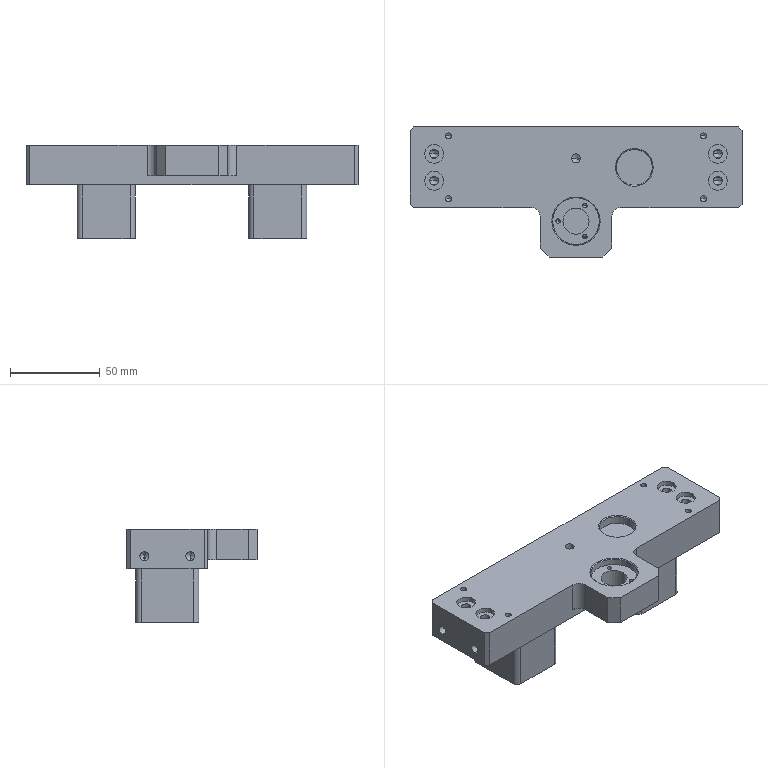NC program | NX | posted with a generic post | part box 185 x 72.5 x 52 mm
Lines 6548 to 6926 of 6926:
(ZLEVEL_PROFILE_COPY_1_COPY_COPY_1 , TOOL : D10JING)
N13076 T14 M6
N13078 G54
N13080 G17 G0 G90 X-32.847 Y-38.112 S9500 M3
N13082 G43 Z30. H14
N13084 Z-13.5
N13086 G94 G1 Z-14.5 F1000.
N13088 X-33.634 Y-36.75
N13090 G3 X-34.5 Y-36.25 R1.
N13092 G1 X-61. F1200.
N13094 G2 X-69. Y-28.25 R8.
N13096 G1 Y0.75
N13098 G2 X-61. Y8.75 R8.
N13100 G1 X-34.5
N13102 G2 X-26.5 Y0.75 R8.
N13104 G1 Y-28.25
N13106 G2 X-34.5 Y-36.25 R8.
N13108 G3 X-35.366 Y-36.75 R1.
N13110 G1 X-36.232 Y-38.25
N13112 Z-13.5
N13114 G0 Z30.
N13116 X-32.847 Y-38.112
N13118 Z-28.
N13120 G1 Z-29. F1000.
N13122 X-33.634 Y-36.75
N13124 G3 X-34.5 Y-36.25 R1.
N13126 G1 X-61. F1200.
N13128 G2 X-69. Y-28.25 R8.
N13130 G1 Y0.75
N13132 G2 X-61. Y8.75 R8.
N13134 G1 X-34.5
N13136 G2 X-26.5 Y0.75 R8.
N13138 G1 Y-28.25
N13140 G2 X-34.5 Y-36.25 R8.
N13142 G3 X-35.366 Y-36.75 R1.
N13144 G1 X-36.232 Y-38.25
N13146 Z-28.
N13148 G0 Z30.
N13150 X62.653 Y-38.112
N13152 Z-13.5
N13154 G1 Z-14.5 F1000.
N13156 X61.866 Y-36.75
N13158 G3 X61. Y-36.25 R1.
N13160 G1 X34.5 F1200.
N13162 G2 X26.5 Y-28.25 R8.
N13164 G1 Y0.75
N13166 G2 X34.5 Y8.75 R8.
N13168 G1 X61.
N13170 G2 X69. Y0.75 R8.
N13172 G1 Y-28.25
N13174 G2 X61. Y-36.25 R8.
N13176 G3 X60.134 Y-36.75 R1.
N13178 G1 X59.268 Y-38.25
N13180 Z-13.5
N13182 G0 Z30.
N13184 X62.653 Y-38.112
N13186 Z-28.
N13188 G1 Z-29. F1000.
N13190 X61.866 Y-36.75
N13192 G3 X61. Y-36.25 R1.
N13194 G1 X34.5 F1200.
N13196 G2 X26.5 Y-28.25 R8.
N13198 G1 Y0.75
N13200 G2 X34.5 Y8.75 R8.
N13202 G1 X61.
N13204 G2 X69. Y0.75 R8.
N13206 G1 Y-28.25
N13208 G2 X61. Y-36.25 R8.
N13210 G3 X60.134 Y-36.75 R1.
N13212 G1 X59.268 Y-38.25
N13214 Z-28.
N13216 G0 Z30.
(ZLEVEL_PROFILE_COPY_1_COPY_COPY_1_COPY , TOOL : D10JING)
N13218 X92.122 Y-43.059
N13220 Z-51.
N13222 G1 Z-52. F1000.
N13224 X91.366 Y-41.75
N13226 G3 X90.5 Y-41.25 R1.
N13228 G1 X-90.5 F1200.
N13230 G2 X-94.036 Y-39.786 R5.
N13232 G1 X-96.036 Y-37.786
N13234 G2 X-97.5 Y-34.25 R5.
N13236 G1 Y6.75
N13238 G2 X-96.036 Y10.286 R5.
N13240 G1 X-94.036 Y12.286
N13242 G2 X-90.5 Y13.75 R5.
N13244 G1 X-25.
N13246 Y31.25
N13248 G2 X-23.536 Y34.786 R5.
N13250 G1 X-18.536 Y39.786
N13252 G2 X-15. Y41.25 R5.
N13254 G1 X15.
N13256 G2 X18.536 Y39.786 R5.
N13258 G1 X23.536 Y34.786
N13260 G2 X25. Y31.25 R5.
N13262 G1 Y13.75
N13264 X90.5
N13266 G2 X94.036 Y12.286 R5.
N13268 G1 X96.036 Y10.286
N13270 G2 X97.5 Y6.75 R5.
N13272 G1 Y-34.25
N13274 G2 X96.036 Y-37.786 R5.
N13276 G1 X94.036 Y-39.786
N13278 G2 X90.5 Y-41.25 R5.
N13280 G3 X89.634 Y-41.75 R1.
N13282 G1 X88.768 Y-43.25
N13284 Z-51.
N13286 G0 Z30.
(FLOOR_WALL , TOOL : D10JING)
N13288 X93.714 Y-42.229
N13290 Z-28.5
N13292 G1 Z-30. F1250.
N13294 X93.437 Y-41.75
N13296 G3 X92.571 Y-41.25 R1.
N13298 G1 X-92.571
N13300 X-97.171 Y-36.65
N13302 X-62.3
N13304 G2 X-68.603 Y-32.05 R8.5
N13306 G1 X-97.5
N13308 Y-27.45
N13310 X-69.5
N13312 Y-22.85
N13314 X-97.5
N13316 Y-18.25
N13318 X-69.5
N13320 Y-13.65
N13322 X-97.5
N13324 Y-9.05
N13326 X-69.5
N13328 Y-4.45
N13330 X-97.5
N13332 Y0.15
N13334 X-69.5
N13336 Y0.75
N13338 G2 X-68.5 Y4.75 R8.5
N13340 G1 X-97.5
N13342 G3 X-98.366 Y4.25 R1.
N13344 G1 X-99. Y3.152
N13346 Z-28.5
N13348 G0 Z30.
N13350 X68.271 Y-36.65
N13352 Z-28.4
N13354 G1 X62.3 Z-30.
N13356 X97.171
N13358 X97.5 Y-36.321
N13360 Y-32.05
N13362 X68.603
N13364 G3 X69.5 Y-28.25 R8.5
N13366 G1 Y-27.45
N13368 X97.5
N13370 Y-22.85
N13372 X69.5
N13374 Y-18.25
N13376 X97.5
N13378 Y-13.65
N13380 X69.5
N13382 Y-9.05
N13384 X97.5
N13386 Y-4.45
N13388 X69.5
N13390 Y0.15
N13392 X97.5
N13394 Y4.75
N13396 X68.5
N13398 G3 X69.349 Y4.221 R1.
N13400 G1 Z-28.5
N13402 G0 Z30.
N13404 X-62.3 Y-36.65
N13406 Z-28.5
N13408 G1 Z-30.
N13410 G3 X-61. Y-36.75 R8.5
N13412 G1 X-34.5
N13414 G3 X-33.2 Y-36.65 R8.5
N13416 G1 X33.2
N13418 G2 X26.897 Y-32.05 R8.5
N13420 G1 X-26.897
N13422 G3 X-26. Y-28.25 R8.5
N13424 G1 Y-27.45
N13426 X26.
N13428 Y-22.85
N13430 X-26.
N13432 Y-18.25
N13434 X26.
N13436 Y-13.65
N13438 X-26.
N13440 Y-9.05
N13442 X26.
N13444 Y-4.45
N13446 X-26.
N13448 Y0.15
N13450 X26.
N13452 Y0.75
N13454 G2 X27. Y4.75 R8.5
N13456 G1 X-27.
N13458 G3 X-26.151 Y4.221 R1.
N13460 G1 Z-28.5
N13462 G0 Z30.
N13464 X-99. Y6.836
N13466 Z-28.5
N13468 G1 Z-30.
N13470 X-97.837 Y8.85
N13472 G2 X-96.971 Y9.35 R1.
N13474 G1 X96.971
N13476 G2 X97.837 Y8.85 R1.
N13478 G1 X99. Y6.836
N13480 Z-28.5
N13482 G0 Z30.
N13484 X71. Y-12.018
N13486 Z-28.5
N13488 G1 Z-30.
N13490 X69.5 Y-12.884
N13492 G3 X69. Y-13.75 R1.
N13494 G1 Y-28.25
N13496 G2 X61. Y-36.25 R8.
N13498 G1 X34.5
N13500 G2 X26.5 Y-28.25 R8.
N13502 G1 Y0.75
N13504 G2 X34.5 Y8.75 R8.
N13506 G1 X61.
N13508 G2 X69. Y0.75 R8.
N13510 G1 Y-13.75
N13512 G3 X69.5 Y-14.616 R1.
N13514 G1 X71. Y-15.482
N13516 Z-28.5
N13518 G0 Z30.
N13520 X-24.5 Y-12.018
N13522 Z-28.5
N13524 G1 Z-30.
N13526 X-26. Y-12.884
N13528 G3 X-26.5 Y-13.75 R1.
N13530 G1 Y-28.25
N13532 G2 X-34.5 Y-36.25 R8.
N13534 G1 X-61.
N13536 G2 X-69. Y-28.25 R8.
N13538 G1 Y0.75
N13540 G2 X-61. Y8.75 R8.
N13542 G1 X-34.5
N13544 G2 X-26.5 Y0.75 R8.
N13546 G1 Y-13.75
N13548 G3 X-26. Y-14.616 R1.
N13550 G1 X-24.5 Y-15.482
N13552 Z-28.5
N13554 G0 Z30.
N13556 X-18.214 Y42.229
N13558 Z-33.5
N13560 G1 Z-35.
N13562 X-17.937 Y41.75
N13564 G3 X-17.071 Y41.25 R1.
N13566 G1 X17.071
N13568 X21.571 Y36.75
N13570 X-21.571
N13572 X-25. Y33.321
N13574 Y32.25
N13576 X25.
N13578 Y27.75
N13580 X-25.
N13582 Y23.25
N13584 X25.
N13586 Y18.75
N13588 X-25.
N13590 Y14.25
N13592 X25.
N13594 G3 X25.866 Y14.75 R1.
N13596 G1 X26.5 Y15.848
N13598 Z-33.5
N13600 G0 Z30.
N13602 X-26.5 Y15.348
N13604 Z-33.5
N13606 G1 Z-35.
N13608 X-25.866 Y14.25
N13610 G3 X-25. Y13.75 R1.
N13612 G1 X24.97
N13614 G3 X25.836 Y14.25 R1.
N13616 G1 X26.5 Y15.4
N13618 Z-33.5
N13620 G0 Z30.
N13622 M5
(PLANAR_MILL_COPY_COPY_COPY_COPY_COPY_COPY_1 , TOOL : D6A45)
N13624 T01 M6
N13626 G54
N13628 G17 G0 G90 X66.1 Y-12.48 S9500 M3
N13630 G43 Z30. H1
N13632 Z0.5
N13634 G94 G1 Z-1. F1250.
N13636 X65.4 Y-12.884
N13638 G3 X64.9 Y-13.75 R1.
N13640 G1 Y-28.25
N13642 G2 X61. Y-32.15 R3.9
N13644 G1 X34.5
N13646 G2 X30.6 Y-28.25 R3.9
N13648 G1 Y0.75
N13650 G2 X34.5 Y4.65 R3.9
N13652 G1 X61.
N13654 G2 X64.9 Y0.75 R3.9
N13656 G1 Y-13.75
N13658 G3 X65.4 Y-14.616 R1.
N13660 G1 X66.1 Y-15.02
N13662 Z0.5
N13664 G0 Z30.
N13666 X-49.02 Y5.85
N13668 Z0.5
N13670 G1 Z-1.
N13672 X-48.616 Y5.15
N13674 G3 X-47.75 Y4.65 R1.
N13676 G1 X-34.5
N13678 G2 X-30.6 Y0.75 R3.9
N13680 G1 Y-28.25
N13682 G2 X-34.5 Y-32.15 R3.9
N13684 G1 X-61.
N13686 G2 X-64.9 Y-28.25 R3.9
N13688 G1 Y0.75
N13690 G2 X-61. Y4.65 R3.9
N13692 G1 X-47.75
N13694 G3 X-46.884 Y5.15 R1.
N13696 G1 X-46.48 Y5.85
N13698 Z0.5
N13700 G0 Z30.
(PLANAR_MILL_COPY_COPY_COPY_COPY_COPY_COPY_1_COPY , TOOL : D6A45)
N13702 X1.27 Y-38.35
N13704 Z-29.5
N13706 G1 Z-31.
N13708 X0.866 Y-37.65
N13710 G3 X0. Y-37.15 R1.
N13712 G1 X-90.459
N13714 G2 X-91.166 Y-36.857 R1.
N13716 G1 X-93.107 Y-34.916
N13718 G2 X-93.4 Y-34.209 R1.
N13720 G1 Y6.709
N13722 G2 X-93.107 Y7.416 R1.
N13724 G1 X-91.166 Y9.357
N13726 G2 X-90.459 Y9.65 R1.
N13728 G1 X90.459
N13730 G2 X91.166 Y9.357 R1.
N13732 G1 X93.107 Y7.416
N13734 G2 X93.4 Y6.709 R1.
N13736 G1 Y-34.209
N13738 G2 X93.107 Y-34.916 R1.
N13740 G1 X91.166 Y-36.857
N13742 G2 X90.459 Y-37.15 R1.
N13744 G1 X0.
N13746 G3 X-0.866 Y-37.65 R1.
N13748 G1 X-1.27 Y-38.35
N13750 Z-29.5
N13752 G0 Z30.
(PLANAR_MILL_COPY_COPY_COPY_COPY_COPY_COPY_1_COPY_COPY , TOOL : D6A45)
N13754 X-22.454 Y13.45
N13756 Z-34.5
N13758 G1 Z-36.
N13760 X-22.05 Y12.75
N13762 G3 X-21.184 Y12.25 R1.
N13764 X-20.9 Y13.75 R4.1
N13766 G1 Y31.209
N13768 G2 X-20.607 Y31.916 R1.
N13770 G1 X-15.666 Y36.857
N13772 G2 X-14.959 Y37.15 R1.
N13774 G1 X14.959
N13776 G2 X15.666 Y36.857 R1.
N13778 G1 X20.607 Y31.916
N13780 G2 X20.9 Y31.209 R1.
N13782 G1 Y13.75
N13784 G3 X21.184 Y12.25 R4.1
N13786 X22.05 Y12.75 R1.
N13788 G1 X22.454 Y13.45
N13790 Z-34.5
N13792 G0 Z30.
N13794 M5
N13796 M2